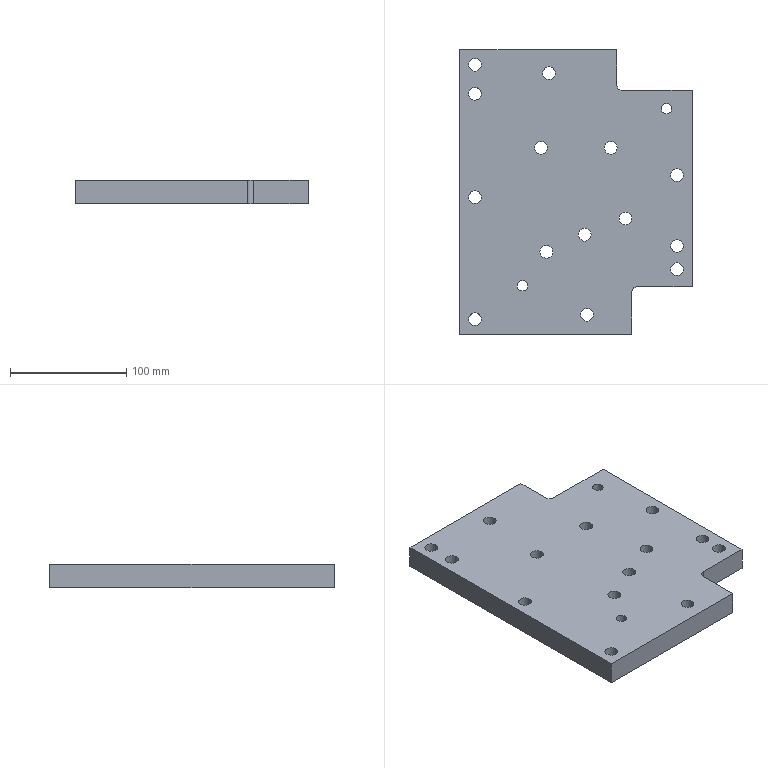Part | STEP file | 114_id2334_x_t | 1 solid | 28 faces | box 200 x 245 x 20 mm | volume 862921 mm3 | cylinder 18 | plane 10 | commonest cylinder face diameters 11 x14 9 x2 10 x2